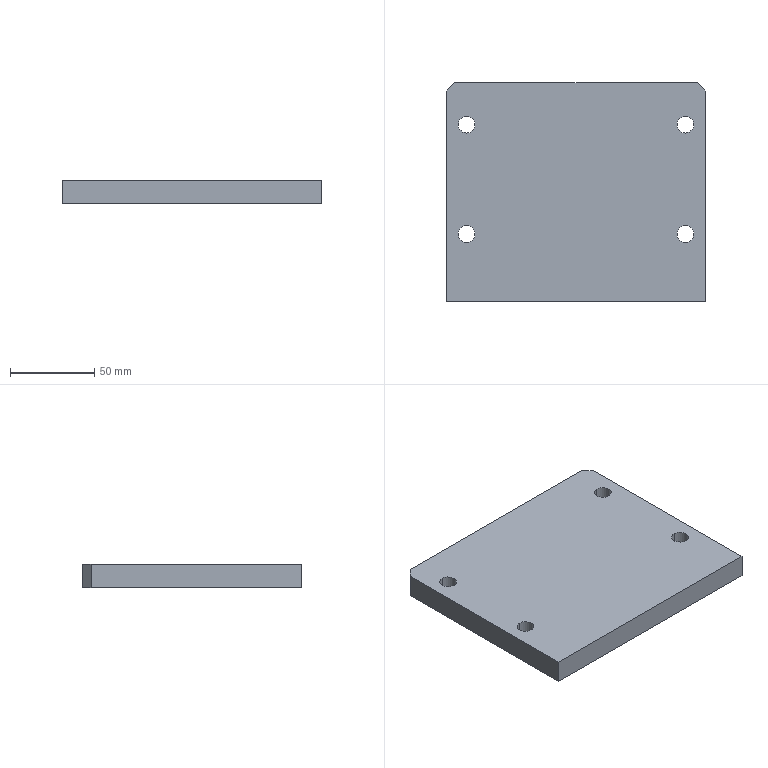Part | STEP file | [01] | 1 solid | 16 faces | box 154 x 130 x 14 mm | volume 275532 mm3 | cylinder 8 | plane 8 | commonest cylinder face diameters 10 x8
STEP:
#1=CARTESIAN_POINT('',(15.,100.,0.));
#2=VERTEX_POINT('',#1);
#3=CARTESIAN_POINT('',(15.,110.,0.));
#4=VERTEX_POINT('',#3);
#5=CARTESIAN_POINT('',(15.,105.,0.));
#6=DIRECTION('',(0.,0.,1.));
#7=DIRECTION('',(0.,1.,0.));
#8=AXIS2_PLACEMENT_3D('',#5,#6,#7);
#9=CIRCLE('',#8,5.);
#10=EDGE_CURVE('',#2,#4,#9,.T.);
#11=ORIENTED_EDGE('',*,*,#10,.F.);
#12=CARTESIAN_POINT('',(15.,100.,14.));
#13=VERTEX_POINT('',#12);
#14=CARTESIAN_POINT('',(15.,100.,0.));
#15=DIRECTION('',(0.,0.,1.));
#16=VECTOR('',#15,1000.);
#17=LINE('',#14,#16);
#18=EDGE_CURVE('',#2,#13,#17,.T.);
#19=ORIENTED_EDGE('',*,*,#18,.T.);
#20=CARTESIAN_POINT('',(15.,110.,14.));
#21=VERTEX_POINT('',#20);
#22=CARTESIAN_POINT('',(15.,105.,14.));
#23=DIRECTION('',(0.,0.,-1.));
#24=DIRECTION('',(0.,-1.,0.));
#25=AXIS2_PLACEMENT_3D('',#22,#23,#24);
#26=CIRCLE('',#25,5.);
#27=EDGE_CURVE('',#21,#13,#26,.T.);
#28=ORIENTED_EDGE('',*,*,#27,.F.);
#29=CARTESIAN_POINT('',(15.,110.,0.));
#30=DIRECTION('',(0.,0.,1.));
#31=VECTOR('',#30,1000.);
#32=LINE('',#29,#31);
#33=EDGE_CURVE('',#4,#21,#32,.T.);
#34=ORIENTED_EDGE('',*,*,#33,.F.);
#35=EDGE_LOOP('',(#11,#19,#28,#34));
#36=FACE_OUTER_BOUND('',#35,.T.);
#37=CARTESIAN_POINT('',(15.,105.,0.));
#38=DIRECTION('',(0.,0.,1.));
#39=DIRECTION('',(0.,1.,0.));
#40=AXIS2_PLACEMENT_3D('',#37,#38,#39);
#41=CYLINDRICAL_SURFACE('',#40,5.);
#42=ADVANCED_FACE('',(#36),#41,.F.);
#43=CARTESIAN_POINT('',(15.,35.,0.));
#44=VERTEX_POINT('',#43);
#45=CARTESIAN_POINT('',(15.,45.,0.));
#46=VERTEX_POINT('',#45);
#47=CARTESIAN_POINT('',(15.,40.,0.));
#48=DIRECTION('',(0.,0.,1.));
#49=DIRECTION('',(0.,1.,0.));
#50=AXIS2_PLACEMENT_3D('',#47,#48,#49);
#51=CIRCLE('',#50,5.);
#52=EDGE_CURVE('',#44,#46,#51,.T.);
#53=ORIENTED_EDGE('',*,*,#52,.F.);
#54=CARTESIAN_POINT('',(15.,35.,14.));
#55=VERTEX_POINT('',#54);
#56=CARTESIAN_POINT('',(15.,35.,0.));
#57=DIRECTION('',(0.,0.,1.));
#58=VECTOR('',#57,1000.);
#59=LINE('',#56,#58);
#60=EDGE_CURVE('',#44,#55,#59,.T.);
#61=ORIENTED_EDGE('',*,*,#60,.T.);
#62=CARTESIAN_POINT('',(15.,45.,14.));
#63=VERTEX_POINT('',#62);
#64=CARTESIAN_POINT('',(15.,40.,14.));
#65=DIRECTION('',(0.,0.,-1.));
#66=DIRECTION('',(0.,-1.,0.));
#67=AXIS2_PLACEMENT_3D('',#64,#65,#66);
#68=CIRCLE('',#67,5.);
#69=EDGE_CURVE('',#63,#55,#68,.T.);
#70=ORIENTED_EDGE('',*,*,#69,.F.);
#71=CARTESIAN_POINT('',(15.,45.,0.));
#72=DIRECTION('',(0.,0.,1.));
#73=VECTOR('',#72,1000.);
#74=LINE('',#71,#73);
#75=EDGE_CURVE('',#46,#63,#74,.T.);
#76=ORIENTED_EDGE('',*,*,#75,.F.);
#77=EDGE_LOOP('',(#53,#61,#70,#76));
#78=FACE_OUTER_BOUND('',#77,.T.);
#79=CARTESIAN_POINT('',(15.,40.,0.));
#80=DIRECTION('',(0.,0.,1.));
#81=DIRECTION('',(0.,1.,0.));
#82=AXIS2_PLACEMENT_3D('',#79,#80,#81);
#83=CYLINDRICAL_SURFACE('',#82,5.);
#84=ADVANCED_FACE('',(#78),#83,.F.);
#85=CARTESIAN_POINT('',(145.,100.,0.));
#86=VERTEX_POINT('',#85);
#87=CARTESIAN_POINT('',(145.,110.,0.));
#88=VERTEX_POINT('',#87);
#89=CARTESIAN_POINT('',(145.,105.,0.));
#90=DIRECTION('',(0.,0.,1.));
#91=DIRECTION('',(0.,1.,0.));
#92=AXIS2_PLACEMENT_3D('',#89,#90,#91);
#93=CIRCLE('',#92,5.);
#94=EDGE_CURVE('',#86,#88,#93,.T.);
#95=ORIENTED_EDGE('',*,*,#94,.F.);
#96=CARTESIAN_POINT('',(145.,100.,14.));
#97=VERTEX_POINT('',#96);
#98=CARTESIAN_POINT('',(145.,100.,0.));
#99=DIRECTION('',(0.,0.,1.));
#100=VECTOR('',#99,1000.);
#101=LINE('',#98,#100);
#102=EDGE_CURVE('',#86,#97,#101,.T.);
#103=ORIENTED_EDGE('',*,*,#102,.T.);
#104=CARTESIAN_POINT('',(145.,110.,14.));
#105=VERTEX_POINT('',#104);
#106=CARTESIAN_POINT('',(145.,105.,14.));
#107=DIRECTION('',(0.,0.,-1.));
#108=DIRECTION('',(0.,-1.,0.));
#109=AXIS2_PLACEMENT_3D('',#106,#107,#108);
#110=CIRCLE('',#109,5.);
#111=EDGE_CURVE('',#105,#97,#110,.T.);
#112=ORIENTED_EDGE('',*,*,#111,.F.);
#113=CARTESIAN_POINT('',(145.,110.,0.));
#114=DIRECTION('',(0.,0.,1.));
#115=VECTOR('',#114,1000.);
#116=LINE('',#113,#115);
#117=EDGE_CURVE('',#88,#105,#116,.T.);
#118=ORIENTED_EDGE('',*,*,#117,.F.);
#119=EDGE_LOOP('',(#95,#103,#112,#118));
#120=FACE_OUTER_BOUND('',#119,.T.);
#121=CARTESIAN_POINT('',(145.,105.,0.));
#122=DIRECTION('',(0.,0.,1.));
#123=DIRECTION('',(0.,1.,0.));
#124=AXIS2_PLACEMENT_3D('',#121,#122,#123);
#125=CYLINDRICAL_SURFACE('',#124,5.);
#126=ADVANCED_FACE('',(#120),#125,.F.);
#127=CARTESIAN_POINT('',(145.,35.,0.));
#128=VERTEX_POINT('',#127);
#129=CARTESIAN_POINT('',(145.,45.,0.));
#130=VERTEX_POINT('',#129);
#131=CARTESIAN_POINT('',(145.,40.,0.));
#132=DIRECTION('',(0.,0.,1.));
#133=DIRECTION('',(0.,1.,0.));
#134=AXIS2_PLACEMENT_3D('',#131,#132,#133);
#135=CIRCLE('',#134,5.);
#136=EDGE_CURVE('',#128,#130,#135,.T.);
#137=ORIENTED_EDGE('',*,*,#136,.F.);
#138=CARTESIAN_POINT('',(145.,35.,14.));
#139=VERTEX_POINT('',#138);
#140=CARTESIAN_POINT('',(145.,35.,0.));
#141=DIRECTION('',(0.,0.,1.));
#142=VECTOR('',#141,1000.);
#143=LINE('',#140,#142);
#144=EDGE_CURVE('',#128,#139,#143,.T.);
#145=ORIENTED_EDGE('',*,*,#144,.T.);
#146=CARTESIAN_POINT('',(145.,45.,14.));
#147=VERTEX_POINT('',#146);
#148=CARTESIAN_POINT('',(145.,40.,14.));
#149=DIRECTION('',(0.,0.,-1.));
#150=DIRECTION('',(0.,-1.,0.));
#151=AXIS2_PLACEMENT_3D('',#148,#149,#150);
#152=CIRCLE('',#151,5.);
#153=EDGE_CURVE('',#147,#139,#152,.T.);
#154=ORIENTED_EDGE('',*,*,#153,.F.);
#155=CARTESIAN_POINT('',(145.,45.,0.));
#156=DIRECTION('',(0.,0.,1.));
#157=VECTOR('',#156,1000.);
#158=LINE('',#155,#157);
#159=EDGE_CURVE('',#130,#147,#158,.T.);
#160=ORIENTED_EDGE('',*,*,#159,.F.);
#161=EDGE_LOOP('',(#137,#145,#154,#160));
#162=FACE_OUTER_BOUND('',#161,.T.);
#163=CARTESIAN_POINT('',(145.,40.,0.));
#164=DIRECTION('',(0.,0.,1.));
#165=DIRECTION('',(0.,1.,0.));
#166=AXIS2_PLACEMENT_3D('',#163,#164,#165);
#167=CYLINDRICAL_SURFACE('',#166,5.);
#168=ADVANCED_FACE('',(#162),#167,.F.);
#169=CARTESIAN_POINT('',(15.,105.,0.));
#170=DIRECTION('',(0.,0.,1.));
#171=DIRECTION('',(0.,1.,0.));
#172=AXIS2_PLACEMENT_3D('',#169,#170,#171);
#173=CIRCLE('',#172,5.);
#174=EDGE_CURVE('',#4,#2,#173,.T.);
#175=ORIENTED_EDGE('',*,*,#174,.T.);
#176=ORIENTED_EDGE('',*,*,#10,.T.);
#177=EDGE_LOOP('',(#175,#176));
#178=FACE_BOUND('',#177,.T.);
#179=CARTESIAN_POINT('',(15.,40.,0.));
#180=DIRECTION('',(0.,0.,1.));
#181=DIRECTION('',(0.,1.,0.));
#182=AXIS2_PLACEMENT_3D('',#179,#180,#181);
#183=CIRCLE('',#182,5.);
#184=EDGE_CURVE('',#46,#44,#183,.T.);
#185=ORIENTED_EDGE('',*,*,#184,.T.);
#186=ORIENTED_EDGE('',*,*,#52,.T.);
#187=EDGE_LOOP('',(#185,#186));
#188=FACE_BOUND('',#187,.T.);
#189=CARTESIAN_POINT('',(145.,105.,0.));
#190=DIRECTION('',(0.,0.,1.));
#191=DIRECTION('',(0.,1.,0.));
#192=AXIS2_PLACEMENT_3D('',#189,#190,#191);
#193=CIRCLE('',#192,5.);
#194=EDGE_CURVE('',#88,#86,#193,.T.);
#195=ORIENTED_EDGE('',*,*,#194,.T.);
#196=ORIENTED_EDGE('',*,*,#94,.T.);
#197=EDGE_LOOP('',(#195,#196));
#198=FACE_BOUND('',#197,.T.);
#199=CARTESIAN_POINT('',(145.,40.,0.));
#200=DIRECTION('',(0.,0.,1.));
#201=DIRECTION('',(0.,1.,0.));
#202=AXIS2_PLACEMENT_3D('',#199,#200,#201);
#203=CIRCLE('',#202,5.);
#204=EDGE_CURVE('',#130,#128,#203,.T.);
#205=ORIENTED_EDGE('',*,*,#204,.T.);
#206=ORIENTED_EDGE('',*,*,#136,.T.);
#207=EDGE_LOOP('',(#205,#206));
#208=FACE_BOUND('',#207,.T.);
#209=CARTESIAN_POINT('',(3.,125.,0.));
#210=VERTEX_POINT('',#209);
#211=CARTESIAN_POINT('',(3.,0.,0.));
#212=VERTEX_POINT('',#211);
#213=CARTESIAN_POINT('',(3.,65.,0.));
#214=DIRECTION('',(0.,-1.,0.));
#215=VECTOR('',#214,1000.);
#216=LINE('',#213,#215);
#217=EDGE_CURVE('',#210,#212,#216,.T.);
#218=ORIENTED_EDGE('',*,*,#217,.F.);
#219=CARTESIAN_POINT('',(8.,130.,0.));
#220=VERTEX_POINT('',#219);
#221=CARTESIAN_POINT('',(11.5,133.5,0.));
#222=DIRECTION('',(0.7071,0.7071,0.));
#223=VECTOR('',#222,1000.);
#224=LINE('',#221,#223);
#225=EDGE_CURVE('',#210,#220,#224,.T.);
#226=ORIENTED_EDGE('',*,*,#225,.T.);
#227=CARTESIAN_POINT('',(152.,130.,0.));
#228=VERTEX_POINT('',#227);
#229=CARTESIAN_POINT('',(80.,130.,0.));
#230=DIRECTION('',(-1.,0.,0.));
#231=VECTOR('',#230,1000.);
#232=LINE('',#229,#231);
#233=EDGE_CURVE('',#228,#220,#232,.T.);
#234=ORIENTED_EDGE('',*,*,#233,.F.);
#235=CARTESIAN_POINT('',(157.,125.,0.));
#236=VERTEX_POINT('',#235);
#237=CARTESIAN_POINT('',(148.5,133.5,0.));
#238=DIRECTION('',(0.7071,-0.7071,0.));
#239=VECTOR('',#238,1000.);
#240=LINE('',#237,#239);
#241=EDGE_CURVE('',#228,#236,#240,.T.);
#242=ORIENTED_EDGE('',*,*,#241,.T.);
#243=CARTESIAN_POINT('',(157.,0.,0.));
#244=VERTEX_POINT('',#243);
#245=CARTESIAN_POINT('',(157.,65.,0.));
#246=DIRECTION('',(0.,1.,0.));
#247=VECTOR('',#246,1000.);
#248=LINE('',#245,#247);
#249=EDGE_CURVE('',#244,#236,#248,.T.);
#250=ORIENTED_EDGE('',*,*,#249,.F.);
#251=CARTESIAN_POINT('',(80.,0.,0.));
#252=DIRECTION('',(1.,0.,0.));
#253=VECTOR('',#252,1000.);
#254=LINE('',#251,#253);
#255=EDGE_CURVE('',#212,#244,#254,.T.);
#256=ORIENTED_EDGE('',*,*,#255,.F.);
#257=EDGE_LOOP('',(#218,#226,#234,#242,#250,#256));
#258=FACE_OUTER_BOUND('',#257,.T.);
#259=CARTESIAN_POINT('',(80.,65.,0.));
#260=DIRECTION('',(0.,0.,-1.));
#261=DIRECTION('',(0.,-1.,0.));
#262=AXIS2_PLACEMENT_3D('',#259,#260,#261);
#263=PLANE('',#262);
#264=ADVANCED_FACE('',(#178,#188,#198,#208,#258),#263,.T.);
#265=ORIENTED_EDGE('',*,*,#249,.T.);
#266=CARTESIAN_POINT('',(157.,125.,14.));
#267=VERTEX_POINT('',#266);
#268=CARTESIAN_POINT('',(157.,125.,14.));
#269=DIRECTION('',(0.,0.,1.));
#270=VECTOR('',#269,1000.);
#271=LINE('',#268,#270);
#272=EDGE_CURVE('',#236,#267,#271,.T.);
#273=ORIENTED_EDGE('',*,*,#272,.T.);
#274=CARTESIAN_POINT('',(157.,0.,14.));
#275=VERTEX_POINT('',#274);
#276=CARTESIAN_POINT('',(157.,65.,14.));
#277=DIRECTION('',(0.,-1.,0.));
#278=VECTOR('',#277,1000.);
#279=LINE('',#276,#278);
#280=EDGE_CURVE('',#267,#275,#279,.T.);
#281=ORIENTED_EDGE('',*,*,#280,.T.);
#282=CARTESIAN_POINT('',(157.,0.,14.));
#283=DIRECTION('',(0.,0.,-1.));
#284=VECTOR('',#283,1000.);
#285=LINE('',#282,#284);
#286=EDGE_CURVE('',#275,#244,#285,.T.);
#287=ORIENTED_EDGE('',*,*,#286,.T.);
#288=EDGE_LOOP('',(#265,#273,#281,#287));
#289=FACE_OUTER_BOUND('',#288,.T.);
#290=CARTESIAN_POINT('',(157.,65.,14.));
#291=DIRECTION('',(1.,0.,0.));
#292=DIRECTION('',(0.,0.,1.));
#293=AXIS2_PLACEMENT_3D('',#290,#291,#292);
#294=PLANE('',#293);
#295=ADVANCED_FACE('',(#289),#294,.T.);
#296=ORIENTED_EDGE('',*,*,#233,.T.);
#297=CARTESIAN_POINT('',(8.,130.,14.));
#298=VERTEX_POINT('',#297);
#299=CARTESIAN_POINT('',(8.,130.,14.));
#300=DIRECTION('',(0.,0.,1.));
#301=VECTOR('',#300,1000.);
#302=LINE('',#299,#301);
#303=EDGE_CURVE('',#220,#298,#302,.T.);
#304=ORIENTED_EDGE('',*,*,#303,.T.);
#305=CARTESIAN_POINT('',(152.,130.,14.));
#306=VERTEX_POINT('',#305);
#307=CARTESIAN_POINT('',(80.,130.,14.));
#308=DIRECTION('',(1.,0.,0.));
#309=VECTOR('',#308,1000.);
#310=LINE('',#307,#309);
#311=EDGE_CURVE('',#298,#306,#310,.T.);
#312=ORIENTED_EDGE('',*,*,#311,.T.);
#313=CARTESIAN_POINT('',(152.,130.,14.));
#314=DIRECTION('',(0.,0.,-1.));
#315=VECTOR('',#314,1000.);
#316=LINE('',#313,#315);
#317=EDGE_CURVE('',#306,#228,#316,.T.);
#318=ORIENTED_EDGE('',*,*,#317,.T.);
#319=EDGE_LOOP('',(#296,#304,#312,#318));
#320=FACE_OUTER_BOUND('',#319,.T.);
#321=CARTESIAN_POINT('',(80.,130.,14.));
#322=DIRECTION('',(0.,1.,0.));
#323=DIRECTION('',(0.,0.,-1.));
#324=AXIS2_PLACEMENT_3D('',#321,#322,#323);
#325=PLANE('',#324);
#326=ADVANCED_FACE('',(#320),#325,.T.);
#327=CARTESIAN_POINT('',(3.,0.,14.));
#328=VERTEX_POINT('',#327);
#329=CARTESIAN_POINT('',(3.,125.,14.));
#330=VERTEX_POINT('',#329);
#331=CARTESIAN_POINT('',(3.,65.,14.));
#332=DIRECTION('',(0.,1.,0.));
#333=VECTOR('',#332,1000.);
#334=LINE('',#331,#333);
#335=EDGE_CURVE('',#328,#330,#334,.T.);
#336=ORIENTED_EDGE('',*,*,#335,.T.);
#337=CARTESIAN_POINT('',(3.,125.,14.));
#338=DIRECTION('',(0.,0.,-1.));
#339=VECTOR('',#338,1000.);
#340=LINE('',#337,#339);
#341=EDGE_CURVE('',#330,#210,#340,.T.);
#342=ORIENTED_EDGE('',*,*,#341,.T.);
#343=ORIENTED_EDGE('',*,*,#217,.T.);
#344=CARTESIAN_POINT('',(3.,0.,14.));
#345=DIRECTION('',(0.,0.,-1.));
#346=VECTOR('',#345,1000.);
#347=LINE('',#344,#346);
#348=EDGE_CURVE('',#328,#212,#347,.T.);
#349=ORIENTED_EDGE('',*,*,#348,.F.);
#350=EDGE_LOOP('',(#336,#342,#343,#349));
#351=FACE_OUTER_BOUND('',#350,.T.);
#352=CARTESIAN_POINT('',(3.,65.,14.));
#353=DIRECTION('',(-1.,0.,0.));
#354=DIRECTION('',(0.,0.,-1.));
#355=AXIS2_PLACEMENT_3D('',#352,#353,#354);
#356=PLANE('',#355);
#357=ADVANCED_FACE('',(#351),#356,.T.);
#358=ORIENTED_EDGE('',*,*,#27,.T.);
#359=CARTESIAN_POINT('',(15.,105.,14.));
#360=DIRECTION('',(0.,0.,-1.));
#361=DIRECTION('',(0.,-1.,0.));
#362=AXIS2_PLACEMENT_3D('',#359,#360,#361);
#363=CIRCLE('',#362,5.);
#364=EDGE_CURVE('',#13,#21,#363,.T.);
#365=ORIENTED_EDGE('',*,*,#364,.T.);
#366=EDGE_LOOP('',(#358,#365));
#367=FACE_BOUND('',#366,.T.);
#368=ORIENTED_EDGE('',*,*,#69,.T.);
#369=CARTESIAN_POINT('',(15.,40.,14.));
#370=DIRECTION('',(0.,0.,-1.));
#371=DIRECTION('',(0.,-1.,0.));
#372=AXIS2_PLACEMENT_3D('',#369,#370,#371);
#373=CIRCLE('',#372,5.);
#374=EDGE_CURVE('',#55,#63,#373,.T.);
#375=ORIENTED_EDGE('',*,*,#374,.T.);
#376=EDGE_LOOP('',(#368,#375));
#377=FACE_BOUND('',#376,.T.);
#378=ORIENTED_EDGE('',*,*,#111,.T.);
#379=CARTESIAN_POINT('',(145.,105.,14.));
#380=DIRECTION('',(0.,0.,-1.));
#381=DIRECTION('',(0.,-1.,0.));
#382=AXIS2_PLACEMENT_3D('',#379,#380,#381);
#383=CIRCLE('',#382,5.);
#384=EDGE_CURVE('',#97,#105,#383,.T.);
#385=ORIENTED_EDGE('',*,*,#384,.T.);
#386=EDGE_LOOP('',(#378,#385));
#387=FACE_BOUND('',#386,.T.);
#388=ORIENTED_EDGE('',*,*,#153,.T.);
#389=CARTESIAN_POINT('',(145.,40.,14.));
#390=DIRECTION('',(0.,0.,-1.));
#391=DIRECTION('',(0.,-1.,0.));
#392=AXIS2_PLACEMENT_3D('',#389,#390,#391);
#393=CIRCLE('',#392,5.);
#394=EDGE_CURVE('',#139,#147,#393,.T.);
#395=ORIENTED_EDGE('',*,*,#394,.T.);
#396=EDGE_LOOP('',(#388,#395));
#397=FACE_BOUND('',#396,.T.);
#398=ORIENTED_EDGE('',*,*,#311,.F.);
#399=CARTESIAN_POINT('',(11.5,133.5,14.));
#400=DIRECTION('',(-0.7071,-0.7071,0.));
#401=VECTOR('',#400,1000.);
#402=LINE('',#399,#401);
#403=EDGE_CURVE('',#298,#330,#402,.T.);
#404=ORIENTED_EDGE('',*,*,#403,.T.);
#405=ORIENTED_EDGE('',*,*,#335,.F.);
#406=CARTESIAN_POINT('',(80.,0.,14.));
#407=DIRECTION('',(-1.,0.,0.));
#408=VECTOR('',#407,1000.);
#409=LINE('',#406,#408);
#410=EDGE_CURVE('',#275,#328,#409,.T.);
#411=ORIENTED_EDGE('',*,*,#410,.F.);
#412=ORIENTED_EDGE('',*,*,#280,.F.);
#413=CARTESIAN_POINT('',(148.5,133.5,14.));
#414=DIRECTION('',(-0.7071,0.7071,0.));
#415=VECTOR('',#414,1000.);
#416=LINE('',#413,#415);
#417=EDGE_CURVE('',#267,#306,#416,.T.);
#418=ORIENTED_EDGE('',*,*,#417,.T.);
#419=EDGE_LOOP('',(#398,#404,#405,#411,#412,#418));
#420=FACE_OUTER_BOUND('',#419,.T.);
#421=CARTESIAN_POINT('',(80.,65.,14.));
#422=DIRECTION('',(0.,0.,1.));
#423=DIRECTION('',(0.,1.,0.));
#424=AXIS2_PLACEMENT_3D('',#421,#422,#423);
#425=PLANE('',#424);
#426=ADVANCED_FACE('',(#367,#377,#387,#397,#420),#425,.T.);
#427=ORIENTED_EDGE('',*,*,#410,.T.);
#428=ORIENTED_EDGE('',*,*,#348,.T.);
#429=ORIENTED_EDGE('',*,*,#255,.T.);
#430=ORIENTED_EDGE('',*,*,#286,.F.);
#431=EDGE_LOOP('',(#427,#428,#429,#430));
#432=FACE_OUTER_BOUND('',#431,.T.);
#433=CARTESIAN_POINT('',(80.,0.,14.));
#434=DIRECTION('',(0.,-1.,0.));
#435=DIRECTION('',(0.,0.,1.));
#436=AXIS2_PLACEMENT_3D('',#433,#434,#435);
#437=PLANE('',#436);
#438=ADVANCED_FACE('',(#432),#437,.T.);
#439=ORIENTED_EDGE('',*,*,#417,.F.);
#440=ORIENTED_EDGE('',*,*,#272,.F.);
#441=ORIENTED_EDGE('',*,*,#241,.F.);
#442=ORIENTED_EDGE('',*,*,#317,.F.);
#443=EDGE_LOOP('',(#439,#440,#441,#442));
#444=FACE_OUTER_BOUND('',#443,.T.);
#445=CARTESIAN_POINT('',(152.,130.,14.));
#446=DIRECTION('',(-0.7071,-0.7071,0.));
#447=DIRECTION('',(0.,0.,-1.));
#448=AXIS2_PLACEMENT_3D('',#445,#446,#447);
#449=PLANE('',#448);
#450=ADVANCED_FACE('',(#444),#449,.F.);
#451=ORIENTED_EDGE('',*,*,#403,.F.);
#452=ORIENTED_EDGE('',*,*,#303,.F.);
#453=ORIENTED_EDGE('',*,*,#225,.F.);
#454=ORIENTED_EDGE('',*,*,#341,.F.);
#455=EDGE_LOOP('',(#451,#452,#453,#454));
#456=FACE_OUTER_BOUND('',#455,.T.);
#457=CARTESIAN_POINT('',(3.,125.,14.));
#458=DIRECTION('',(0.7071,-0.7071,0.));
#459=DIRECTION('',(0.,0.,-1.));
#460=AXIS2_PLACEMENT_3D('',#457,#458,#459);
#461=PLANE('',#460);
#462=ADVANCED_FACE('',(#456),#461,.F.);
#463=ORIENTED_EDGE('',*,*,#144,.F.);
#464=ORIENTED_EDGE('',*,*,#204,.F.);
#465=ORIENTED_EDGE('',*,*,#159,.T.);
#466=ORIENTED_EDGE('',*,*,#394,.F.);
#467=EDGE_LOOP('',(#463,#464,#465,#466));
#468=FACE_OUTER_BOUND('',#467,.T.);
#469=CARTESIAN_POINT('',(145.,40.,0.));
#470=DIRECTION('',(0.,0.,1.));
#471=DIRECTION('',(0.,1.,0.));
#472=AXIS2_PLACEMENT_3D('',#469,#470,#471);
#473=CYLINDRICAL_SURFACE('',#472,5.);
#474=ADVANCED_FACE('',(#468),#473,.F.);
#475=ORIENTED_EDGE('',*,*,#102,.F.);
#476=ORIENTED_EDGE('',*,*,#194,.F.);
#477=ORIENTED_EDGE('',*,*,#117,.T.);
#478=ORIENTED_EDGE('',*,*,#384,.F.);
#479=EDGE_LOOP('',(#475,#476,#477,#478));
#480=FACE_OUTER_BOUND('',#479,.T.);
#481=CARTESIAN_POINT('',(145.,105.,0.));
#482=DIRECTION('',(0.,0.,1.));
#483=DIRECTION('',(0.,1.,0.));
#484=AXIS2_PLACEMENT_3D('',#481,#482,#483);
#485=CYLINDRICAL_SURFACE('',#484,5.);
#486=ADVANCED_FACE('',(#480),#485,.F.);
#487=ORIENTED_EDGE('',*,*,#60,.F.);
#488=ORIENTED_EDGE('',*,*,#184,.F.);
#489=ORIENTED_EDGE('',*,*,#75,.T.);
#490=ORIENTED_EDGE('',*,*,#374,.F.);
#491=EDGE_LOOP('',(#487,#488,#489,#490));
#492=FACE_OUTER_BOUND('',#491,.T.);
#493=CARTESIAN_POINT('',(15.,40.,0.));
#494=DIRECTION('',(0.,0.,1.));
#495=DIRECTION('',(0.,1.,0.));
#496=AXIS2_PLACEMENT_3D('',#493,#494,#495);
#497=CYLINDRICAL_SURFACE('',#496,5.);
#498=ADVANCED_FACE('',(#492),#497,.F.);
#499=ORIENTED_EDGE('',*,*,#18,.F.);
#500=ORIENTED_EDGE('',*,*,#174,.F.);
#501=ORIENTED_EDGE('',*,*,#33,.T.);
#502=ORIENTED_EDGE('',*,*,#364,.F.);
#503=EDGE_LOOP('',(#499,#500,#501,#502));
#504=FACE_OUTER_BOUND('',#503,.T.);
#505=CARTESIAN_POINT('',(15.,105.,0.));
#506=DIRECTION('',(0.,0.,1.));
#507=DIRECTION('',(0.,1.,0.));
#508=AXIS2_PLACEMENT_3D('',#505,#506,#507);
#509=CYLINDRICAL_SURFACE('',#508,5.);
#510=ADVANCED_FACE('',(#504),#509,.F.);
#511=CLOSED_SHELL('',(#42,#84,#126,#168,#264,#295,#326,#357,#426,#438,#450,#462,#474,#486,#498,#510));
#512=MANIFOLD_SOLID_BREP('',#511);
#513=CARTESIAN_POINT('',(0.,0.,0.));
#514=DIRECTION('',(0.,0.,1.));
#515=DIRECTION('',(1.,0.,0.));
#516=AXIS2_PLACEMENT_3D('',#513,#514,#515);
#517=(LENGTH_UNIT()NAMED_UNIT(*)SI_UNIT(.MILLI.,.METRE.));
#518=UNCERTAINTY_MEASURE_WITH_UNIT(LENGTH_MEASURE(0.00001),#517,'','');
#519=(NAMED_UNIT(*)PLANE_ANGLE_UNIT()SI_UNIT($,.RADIAN.));
#520=(NAMED_UNIT(*)SI_UNIT($,.STERADIAN.)SOLID_ANGLE_UNIT());
#521=(GEOMETRIC_REPRESENTATION_CONTEXT(3)GLOBAL_UNCERTAINTY_ASSIGNED_CONTEXT((#518))GLOBAL_UNIT_ASSIGNED_CONTEXT((#517,#519,#520))REPRESENTATION_CONTEXT('',''));
#522=ADVANCED_BREP_SHAPE_REPRESENTATION('',(#512,#516),#521);